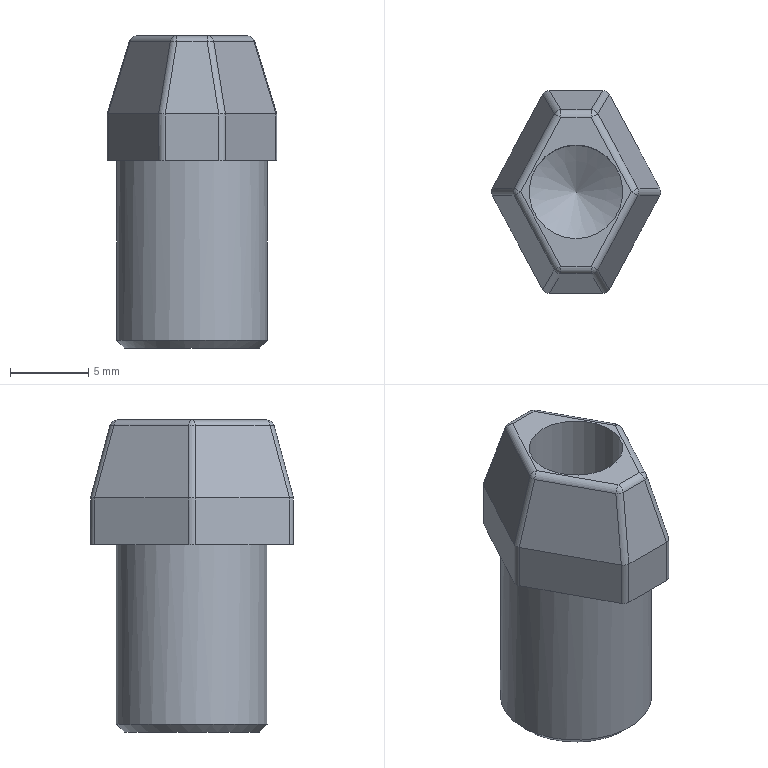Part | NX | features solid 2 | 1 solid | 46 faces | box 10.864 x 13 x 20 mm | volume 1244 mm3 | cylinder 20 | plane 18 | sphere 6 | cone 2 | commonest cylinder face diameters 1 x18 6 x1 9.685 x1
STEP:
#1=CARTESIAN_POINT('',(-137.368,-255.227,120.662));
#2=VERTEX_POINT('',#1);
#3=CARTESIAN_POINT('',(-136.259,-257.286,120.662));
#4=VERTEX_POINT('',#3);
#5=CARTESIAN_POINT('',(-137.495,-254.99,120.662));
#6=DIRECTION('',(0.4741,-0.8805,0.));
#7=VECTOR('',#6,1000.);
#8=LINE('',#5,#7);
#9=EDGE_CURVE('',#2,#4,#8,.T.);
#10=ORIENTED_EDGE('',*,*,#9,.F.);
#11=CARTESIAN_POINT('',(-137.368,-254.753,120.662));
#12=VERTEX_POINT('',#11);
#13=CARTESIAN_POINT('',(-136.927,-254.99,120.662));
#14=DIRECTION('',(0.,0.,1.));
#15=DIRECTION('',(0.,1.,0.));
#16=AXIS2_PLACEMENT_3D('',#13,#14,#15);
#17=CIRCLE('',#16,0.5);
#18=EDGE_CURVE('',#2,#12,#17,.F.);
#19=ORIENTED_EDGE('',*,*,#18,.T.);
#20=CARTESIAN_POINT('',(-136.259,-252.694,120.662));
#21=VERTEX_POINT('',#20);
#22=CARTESIAN_POINT('',(-133.995,-248.49,120.662));
#23=DIRECTION('',(-0.4741,-0.8805,0.));
#24=VECTOR('',#23,1000.);
#25=LINE('',#22,#24);
#26=EDGE_CURVE('',#21,#12,#25,.T.);
#27=ORIENTED_EDGE('',*,*,#26,.F.);
#28=CARTESIAN_POINT('',(-131.995,-254.99,120.662));
#29=DIRECTION('',(0.,0.,1.));
#30=DIRECTION('',(0.,1.,0.));
#31=AXIS2_PLACEMENT_3D('',#28,#29,#30);
#32=CIRCLE('',#31,4.843);
#33=EDGE_CURVE('',#21,#4,#32,.T.);
#34=ORIENTED_EDGE('',*,*,#33,.T.);
#35=EDGE_LOOP('',(#10,#19,#27,#34));
#36=FACE_BOUND('',#35,.T.);
#37=CARTESIAN_POINT('',(-122.995,-261.49,120.662));
#38=DIRECTION('',(0.,0.,1.));
#39=DIRECTION('',(0.,1.,0.));
#40=AXIS2_PLACEMENT_3D('',#37,#38,#39);
#41=PLANE('',#40);
#42=ADVANCED_FACE('',(#36),#41,.F.);
#43=CARTESIAN_POINT('',(-129.854,-261.227,120.662));
#44=VERTEX_POINT('',#43);
#45=CARTESIAN_POINT('',(-127.732,-257.286,120.662));
#46=VERTEX_POINT('',#45);
#47=CARTESIAN_POINT('',(-129.995,-261.49,120.662));
#48=DIRECTION('',(0.4741,0.8805,0.));
#49=VECTOR('',#48,1000.);
#50=LINE('',#47,#49);
#51=EDGE_CURVE('',#44,#46,#50,.T.);
#52=ORIENTED_EDGE('',*,*,#51,.F.);
#53=CARTESIAN_POINT('',(-130.294,-261.49,120.662));
#54=VERTEX_POINT('',#53);
#55=CARTESIAN_POINT('',(-130.294,-260.99,120.662));
#56=DIRECTION('',(0.,0.,1.));
#57=DIRECTION('',(0.,1.,0.));
#58=AXIS2_PLACEMENT_3D('',#55,#56,#57);
#59=CIRCLE('',#58,0.5);
#60=EDGE_CURVE('',#44,#54,#59,.F.);
#61=ORIENTED_EDGE('',*,*,#60,.T.);
#62=CARTESIAN_POINT('',(-133.697,-261.49,120.662));
#63=VERTEX_POINT('',#62);
#64=CARTESIAN_POINT('',(-133.995,-261.49,120.662));
#65=DIRECTION('',(1.,0.,0.));
#66=VECTOR('',#65,1000.);
#67=LINE('',#64,#66);
#68=EDGE_CURVE('',#63,#54,#67,.T.);
#69=ORIENTED_EDGE('',*,*,#68,.F.);
#70=CARTESIAN_POINT('',(-134.137,-261.227,120.662));
#71=VERTEX_POINT('',#70);
#72=CARTESIAN_POINT('',(-133.697,-260.99,120.662));
#73=DIRECTION('',(0.,0.,1.));
#74=DIRECTION('',(0.,1.,0.));
#75=AXIS2_PLACEMENT_3D('',#72,#73,#74);
#76=CIRCLE('',#75,0.5);
#77=EDGE_CURVE('',#63,#71,#76,.F.);
#78=ORIENTED_EDGE('',*,*,#77,.T.);
#79=CARTESIAN_POINT('',(-137.495,-254.99,120.662));
#80=DIRECTION('',(0.4741,-0.8805,0.));
#81=VECTOR('',#80,1000.);
#82=LINE('',#79,#81);
#83=EDGE_CURVE('',#4,#71,#82,.T.);
#84=ORIENTED_EDGE('',*,*,#83,.F.);
#85=CARTESIAN_POINT('',(-131.995,-254.99,120.662));
#86=DIRECTION('',(0.,0.,1.));
#87=DIRECTION('',(0.,1.,0.));
#88=AXIS2_PLACEMENT_3D('',#85,#86,#87);
#89=CIRCLE('',#88,4.843);
#90=EDGE_CURVE('',#4,#46,#89,.T.);
#91=ORIENTED_EDGE('',*,*,#90,.T.);
#92=EDGE_LOOP('',(#52,#61,#69,#78,#84,#91));
#93=FACE_BOUND('',#92,.T.);
#94=CARTESIAN_POINT('',(-122.995,-261.49,120.662));
#95=DIRECTION('',(0.,0.,1.));
#96=DIRECTION('',(0.,1.,0.));
#97=AXIS2_PLACEMENT_3D('',#94,#95,#96);
#98=PLANE('',#97);
#99=ADVANCED_FACE('',(#93),#98,.F.);
#100=CARTESIAN_POINT('',(-126.623,-254.753,120.662));
#101=VERTEX_POINT('',#100);
#102=CARTESIAN_POINT('',(-127.732,-252.694,120.662));
#103=VERTEX_POINT('',#102);
#104=CARTESIAN_POINT('',(-126.495,-254.99,120.662));
#105=DIRECTION('',(-0.4741,0.8805,0.));
#106=VECTOR('',#105,1000.);
#107=LINE('',#104,#106);
#108=EDGE_CURVE('',#101,#103,#107,.T.);
#109=ORIENTED_EDGE('',*,*,#108,.F.);
#110=CARTESIAN_POINT('',(-126.623,-255.227,120.662));
#111=VERTEX_POINT('',#110);
#112=CARTESIAN_POINT('',(-127.063,-254.99,120.662));
#113=DIRECTION('',(0.,0.,1.));
#114=DIRECTION('',(0.,1.,0.));
#115=AXIS2_PLACEMENT_3D('',#112,#113,#114);
#116=CIRCLE('',#115,0.5);
#117=EDGE_CURVE('',#101,#111,#116,.F.);
#118=ORIENTED_EDGE('',*,*,#117,.T.);
#119=CARTESIAN_POINT('',(-129.995,-261.49,120.662));
#120=DIRECTION('',(0.4741,0.8805,0.));
#121=VECTOR('',#120,1000.);
#122=LINE('',#119,#121);
#123=EDGE_CURVE('',#46,#111,#122,.T.);
#124=ORIENTED_EDGE('',*,*,#123,.F.);
#125=CARTESIAN_POINT('',(-131.995,-254.99,120.662));
#126=DIRECTION('',(0.,0.,1.));
#127=DIRECTION('',(0.,1.,0.));
#128=AXIS2_PLACEMENT_3D('',#125,#126,#127);
#129=CIRCLE('',#128,4.843);
#130=EDGE_CURVE('',#46,#103,#129,.T.);
#131=ORIENTED_EDGE('',*,*,#130,.T.);
#132=EDGE_LOOP('',(#109,#118,#124,#131));
#133=FACE_BOUND('',#132,.T.);
#134=CARTESIAN_POINT('',(-122.995,-261.49,120.662));
#135=DIRECTION('',(0.,0.,1.));
#136=DIRECTION('',(0.,1.,0.));
#137=AXIS2_PLACEMENT_3D('',#134,#135,#136);
#138=PLANE('',#137);
#139=ADVANCED_FACE('',(#133),#138,.F.);
#140=ORIENTED_EDGE('',*,*,#68,.T.);
#141=CARTESIAN_POINT('',(-130.294,-261.49,123.662));
#142=VERTEX_POINT('',#141);
#143=CARTESIAN_POINT('',(-130.294,-261.49,123.662));
#144=DIRECTION('',(0.,0.,-1.));
#145=VECTOR('',#144,1000.);
#146=LINE('',#143,#145);
#147=EDGE_CURVE('',#54,#142,#146,.F.);
#148=ORIENTED_EDGE('',*,*,#147,.T.);
#149=CARTESIAN_POINT('',(-133.697,-261.49,123.662));
#150=VERTEX_POINT('',#149);
#151=CARTESIAN_POINT('',(-133.995,-261.49,123.662));
#152=DIRECTION('',(1.,0.,0.));
#153=VECTOR('',#152,1000.);
#154=LINE('',#151,#153);
#155=EDGE_CURVE('',#150,#142,#154,.T.);
#156=ORIENTED_EDGE('',*,*,#155,.F.);
#157=CARTESIAN_POINT('',(-133.697,-261.49,123.662));
#158=DIRECTION('',(0.,0.,-1.));
#159=VECTOR('',#158,1000.);
#160=LINE('',#157,#159);
#161=EDGE_CURVE('',#150,#63,#160,.T.);
#162=ORIENTED_EDGE('',*,*,#161,.T.);
#163=EDGE_LOOP('',(#140,#148,#156,#162));
#164=FACE_BOUND('',#163,.T.);
#165=CARTESIAN_POINT('',(-133.995,-261.49,123.662));
#166=DIRECTION('',(0.,1.,0.));
#167=DIRECTION('',(0.,0.,-1.));
#168=AXIS2_PLACEMENT_3D('',#165,#166,#167);
#169=PLANE('',#168);
#170=ADVANCED_FACE('',(#164),#169,.F.);
#171=ORIENTED_EDGE('',*,*,#123,.T.);
#172=CARTESIAN_POINT('',(-126.623,-255.227,123.662));
#173=VERTEX_POINT('',#172);
#174=CARTESIAN_POINT('',(-126.623,-255.227,123.662));
#175=DIRECTION('',(0.,0.,-1.));
#176=VECTOR('',#175,1000.);
#177=LINE('',#174,#176);
#178=EDGE_CURVE('',#111,#173,#177,.F.);
#179=ORIENTED_EDGE('',*,*,#178,.T.);
#180=CARTESIAN_POINT('',(-129.854,-261.227,123.662));
#181=VERTEX_POINT('',#180);
#182=CARTESIAN_POINT('',(-129.995,-261.49,123.662));
#183=DIRECTION('',(0.4741,0.8805,0.));
#184=VECTOR('',#183,1000.);
#185=LINE('',#182,#184);
#186=EDGE_CURVE('',#181,#173,#185,.T.);
#187=ORIENTED_EDGE('',*,*,#186,.F.);
#188=CARTESIAN_POINT('',(-129.854,-261.227,123.662));
#189=DIRECTION('',(0.,0.,-1.));
#190=VECTOR('',#189,1000.);
#191=LINE('',#188,#190);
#192=EDGE_CURVE('',#181,#44,#191,.T.);
#193=ORIENTED_EDGE('',*,*,#192,.T.);
#194=ORIENTED_EDGE('',*,*,#51,.T.);
#195=EDGE_LOOP('',(#171,#179,#187,#193,#194));
#196=FACE_BOUND('',#195,.T.);
#197=CARTESIAN_POINT('',(-129.995,-261.49,123.662));
#198=DIRECTION('',(-0.8805,0.4741,0.));
#199=DIRECTION('',(-0.4741,-0.8805,0.));
#200=AXIS2_PLACEMENT_3D('',#197,#198,#199);
#201=PLANE('',#200);
#202=ADVANCED_FACE('',(#196),#201,.F.);
#203=CARTESIAN_POINT('',(-129.854,-248.753,120.662));
#204=VERTEX_POINT('',#203);
#205=CARTESIAN_POINT('',(-126.495,-254.99,120.662));
#206=DIRECTION('',(-0.4741,0.8805,0.));
#207=VECTOR('',#206,1000.);
#208=LINE('',#205,#207);
#209=EDGE_CURVE('',#103,#204,#208,.T.);
#210=ORIENTED_EDGE('',*,*,#209,.T.);
#211=CARTESIAN_POINT('',(-129.854,-248.753,123.662));
#212=VERTEX_POINT('',#211);
#213=CARTESIAN_POINT('',(-129.854,-248.753,123.662));
#214=DIRECTION('',(0.,0.,-1.));
#215=VECTOR('',#214,1000.);
#216=LINE('',#213,#215);
#217=EDGE_CURVE('',#204,#212,#216,.F.);
#218=ORIENTED_EDGE('',*,*,#217,.T.);
#219=CARTESIAN_POINT('',(-126.623,-254.753,123.662));
#220=VERTEX_POINT('',#219);
#221=CARTESIAN_POINT('',(-126.495,-254.99,123.662));
#222=DIRECTION('',(-0.4741,0.8805,0.));
#223=VECTOR('',#222,1000.);
#224=LINE('',#221,#223);
#225=EDGE_CURVE('',#220,#212,#224,.T.);
#226=ORIENTED_EDGE('',*,*,#225,.F.);
#227=CARTESIAN_POINT('',(-126.623,-254.753,123.662));
#228=DIRECTION('',(0.,0.,-1.));
#229=VECTOR('',#228,1000.);
#230=LINE('',#227,#229);
#231=EDGE_CURVE('',#220,#101,#230,.T.);
#232=ORIENTED_EDGE('',*,*,#231,.T.);
#233=ORIENTED_EDGE('',*,*,#108,.T.);
#234=EDGE_LOOP('',(#210,#218,#226,#232,#233));
#235=FACE_BOUND('',#234,.T.);
#236=CARTESIAN_POINT('',(-126.495,-254.99,123.662));
#237=DIRECTION('',(-0.8805,-0.4741,0.));
#238=DIRECTION('',(0.4741,-0.8805,0.));
#239=AXIS2_PLACEMENT_3D('',#236,#237,#238);
#240=PLANE('',#239);
#241=ADVANCED_FACE('',(#235),#240,.F.);
#242=CARTESIAN_POINT('',(-130.294,-248.49,123.662));
#243=VERTEX_POINT('',#242);
#244=CARTESIAN_POINT('',(-133.697,-248.49,123.662));
#245=VERTEX_POINT('',#244);
#246=CARTESIAN_POINT('',(-129.995,-248.49,123.662));
#247=DIRECTION('',(-1.,0.,0.));
#248=VECTOR('',#247,1000.);
#249=LINE('',#246,#248);
#250=EDGE_CURVE('',#243,#245,#249,.T.);
#251=ORIENTED_EDGE('',*,*,#250,.F.);
#252=CARTESIAN_POINT('',(-130.294,-248.49,120.662));
#253=VERTEX_POINT('',#252);
#254=CARTESIAN_POINT('',(-130.294,-248.49,123.662));
#255=DIRECTION('',(0.,0.,-1.));
#256=VECTOR('',#255,1000.);
#257=LINE('',#254,#256);
#258=EDGE_CURVE('',#243,#253,#257,.T.);
#259=ORIENTED_EDGE('',*,*,#258,.T.);
#260=CARTESIAN_POINT('',(-133.697,-248.49,120.662));
#261=VERTEX_POINT('',#260);
#262=CARTESIAN_POINT('',(-129.995,-248.49,120.662));
#263=DIRECTION('',(-1.,0.,0.));
#264=VECTOR('',#263,1000.);
#265=LINE('',#262,#264);
#266=EDGE_CURVE('',#253,#261,#265,.T.);
#267=ORIENTED_EDGE('',*,*,#266,.T.);
#268=CARTESIAN_POINT('',(-133.697,-248.49,123.662));
#269=DIRECTION('',(0.,0.,-1.));
#270=VECTOR('',#269,1000.);
#271=LINE('',#268,#270);
#272=EDGE_CURVE('',#261,#245,#271,.F.);
#273=ORIENTED_EDGE('',*,*,#272,.T.);
#274=EDGE_LOOP('',(#251,#259,#267,#273));
#275=FACE_BOUND('',#274,.T.);
#276=CARTESIAN_POINT('',(-129.995,-248.49,123.662));
#277=DIRECTION('',(0.,-1.,0.));
#278=DIRECTION('',(0.,0.,1.));
#279=AXIS2_PLACEMENT_3D('',#276,#277,#278);
#280=PLANE('',#279);
#281=ADVANCED_FACE('',(#275),#280,.F.);
#282=ORIENTED_EDGE('',*,*,#26,.T.);
#283=CARTESIAN_POINT('',(-137.368,-254.753,123.662));
#284=VERTEX_POINT('',#283);
#285=CARTESIAN_POINT('',(-137.368,-254.753,123.662));
#286=DIRECTION('',(0.,0.,-1.));
#287=VECTOR('',#286,1000.);
#288=LINE('',#285,#287);
#289=EDGE_CURVE('',#12,#284,#288,.F.);
#290=ORIENTED_EDGE('',*,*,#289,.T.);
#291=CARTESIAN_POINT('',(-134.137,-248.753,123.662));
#292=VERTEX_POINT('',#291);
#293=CARTESIAN_POINT('',(-133.995,-248.49,123.662));
#294=DIRECTION('',(-0.4741,-0.8805,0.));
#295=VECTOR('',#294,1000.);
#296=LINE('',#293,#295);
#297=EDGE_CURVE('',#292,#284,#296,.T.);
#298=ORIENTED_EDGE('',*,*,#297,.F.);
#299=CARTESIAN_POINT('',(-134.137,-248.753,120.662));
#300=VERTEX_POINT('',#299);
#301=CARTESIAN_POINT('',(-134.137,-248.753,123.662));
#302=DIRECTION('',(0.,0.,-1.));
#303=VECTOR('',#302,1000.);
#304=LINE('',#301,#303);
#305=EDGE_CURVE('',#292,#300,#304,.T.);
#306=ORIENTED_EDGE('',*,*,#305,.T.);
#307=CARTESIAN_POINT('',(-133.995,-248.49,120.662));
#308=DIRECTION('',(-0.4741,-0.8805,0.));
#309=VECTOR('',#308,1000.);
#310=LINE('',#307,#309);
#311=EDGE_CURVE('',#300,#21,#310,.T.);
#312=ORIENTED_EDGE('',*,*,#311,.T.);
#313=EDGE_LOOP('',(#282,#290,#298,#306,#312));
#314=FACE_BOUND('',#313,.T.);
#315=CARTESIAN_POINT('',(-133.995,-248.49,123.662));
#316=DIRECTION('',(0.8805,-0.4741,0.));
#317=DIRECTION('',(0.4741,0.8805,0.));
#318=AXIS2_PLACEMENT_3D('',#315,#316,#317);
#319=PLANE('',#318);
#320=ADVANCED_FACE('',(#314),#319,.F.);
#321=ORIENTED_EDGE('',*,*,#83,.T.);
#322=CARTESIAN_POINT('',(-134.137,-261.227,123.662));
#323=VERTEX_POINT('',#322);
#324=CARTESIAN_POINT('',(-134.137,-261.227,123.662));
#325=DIRECTION('',(0.,0.,-1.));
#326=VECTOR('',#325,1000.);
#327=LINE('',#324,#326);
#328=EDGE_CURVE('',#71,#323,#327,.F.);
#329=ORIENTED_EDGE('',*,*,#328,.T.);
#330=CARTESIAN_POINT('',(-137.368,-255.227,123.662));
#331=VERTEX_POINT('',#330);
#332=CARTESIAN_POINT('',(-137.495,-254.99,123.662));
#333=DIRECTION('',(0.4741,-0.8805,0.));
#334=VECTOR('',#333,1000.);
#335=LINE('',#332,#334);
#336=EDGE_CURVE('',#331,#323,#335,.T.);
#337=ORIENTED_EDGE('',*,*,#336,.F.);
#338=CARTESIAN_POINT('',(-137.368,-255.227,123.662));
#339=DIRECTION('',(0.,0.,-1.));
#340=VECTOR('',#339,1000.);
#341=LINE('',#338,#340);
#342=EDGE_CURVE('',#331,#2,#341,.T.);
#343=ORIENTED_EDGE('',*,*,#342,.T.);
#344=ORIENTED_EDGE('',*,*,#9,.T.);
#345=EDGE_LOOP('',(#321,#329,#337,#343,#344));
#346=FACE_BOUND('',#345,.T.);
#347=CARTESIAN_POINT('',(-137.495,-254.99,123.662));
#348=DIRECTION('',(0.8805,0.4741,0.));
#349=DIRECTION('',(-0.4741,0.8805,0.));
#350=AXIS2_PLACEMENT_3D('',#347,#348,#349);
#351=PLANE('',#350);
#352=ADVANCED_FACE('',(#346),#351,.F.);
#353=ORIENTED_EDGE('',*,*,#266,.F.);
#354=CARTESIAN_POINT('',(-130.294,-248.99,120.662));
#355=DIRECTION('',(0.,0.,1.));
#356=DIRECTION('',(0.,1.,0.));
#357=AXIS2_PLACEMENT_3D('',#354,#355,#356);
#358=CIRCLE('',#357,0.5);
#359=EDGE_CURVE('',#253,#204,#358,.F.);
#360=ORIENTED_EDGE('',*,*,#359,.T.);
#361=ORIENTED_EDGE('',*,*,#209,.F.);
#362=CARTESIAN_POINT('',(-131.995,-254.99,120.662));
#363=DIRECTION('',(0.,0.,1.));
#364=DIRECTION('',(0.,1.,0.));
#365=AXIS2_PLACEMENT_3D('',#362,#363,#364);
#366=CIRCLE('',#365,4.843);
#367=EDGE_CURVE('',#103,#21,#366,.T.);
#368=ORIENTED_EDGE('',*,*,#367,.T.);
#369=ORIENTED_EDGE('',*,*,#311,.F.);
#370=CARTESIAN_POINT('',(-133.697,-248.99,120.662));
#371=DIRECTION('',(0.,0.,1.));
#372=DIRECTION('',(0.,1.,0.));
#373=AXIS2_PLACEMENT_3D('',#370,#371,#372);
#374=CIRCLE('',#373,0.5);
#375=EDGE_CURVE('',#300,#261,#374,.F.);
#376=ORIENTED_EDGE('',*,*,#375,.T.);
#377=EDGE_LOOP('',(#353,#360,#361,#368,#369,#376));
#378=FACE_BOUND('',#377,.T.);
#379=CARTESIAN_POINT('',(-122.995,-261.49,120.662));
#380=DIRECTION('',(0.,0.,1.));
#381=DIRECTION('',(0.,1.,0.));
#382=AXIS2_PLACEMENT_3D('',#379,#380,#381);
#383=PLANE('',#382);
#384=ADVANCED_FACE('',(#378),#383,.F.);
#385=ORIENTED_EDGE('',*,*,#336,.T.);
#386=CARTESIAN_POINT('',(-134.132,-261.236,123.663));
#387=VERTEX_POINT('',#386);
#388=CARTESIAN_POINT('',(-133.697,-260.99,125.528));
#389=DIRECTION('',(-0.8505,-0.4579,0.2588));
#390=DIRECTION('',(-0.2279,-0.1227,-0.9659));
#391=AXIS2_PLACEMENT_3D('',#388,#389,#390);
#392=ELLIPSE('',#391,1.932,0.5);
#393=EDGE_CURVE('',#323,#387,#392,.T.);
#394=ORIENTED_EDGE('',*,*,#393,.T.);
#395=CARTESIAN_POINT('',(-133.391,-259.996,128.292));
#396=VERTEX_POINT('',#395);
#397=CARTESIAN_POINT('',(-134.027,-261.061,124.317));
#398=DIRECTION('',(0.1528,0.2558,0.9546));
#399=VECTOR('',#398,1000.);
#400=LINE('',#397,#399);
#401=EDGE_CURVE('',#387,#396,#400,.T.);
#402=ORIENTED_EDGE('',*,*,#401,.T.);
#403=CARTESIAN_POINT('',(-135.963,-255.219,128.292));
#404=VERTEX_POINT('',#403);
#405=CARTESIAN_POINT('',(-136.061,-255.037,128.292));
#406=DIRECTION('',(0.4741,-0.8805,0.));
#407=VECTOR('',#406,1000.);
#408=LINE('',#405,#407);
#409=EDGE_CURVE('',#396,#404,#408,.F.);
#410=ORIENTED_EDGE('',*,*,#409,.T.);
#411=CARTESIAN_POINT('',(-137.372,-255.219,123.663));
#412=VERTEX_POINT('',#411);
#413=CARTESIAN_POINT('',(-137.278,-255.219,123.972));
#414=DIRECTION('',(0.2911,0.,0.9567));
#415=VECTOR('',#414,1000.);
#416=LINE('',#413,#415);
#417=EDGE_CURVE('',#404,#412,#416,.F.);
#418=ORIENTED_EDGE('',*,*,#417,.T.);
#419=CARTESIAN_POINT('',(-136.927,-254.99,125.528));
#420=DIRECTION('',(-0.8505,-0.4579,0.2588));
#421=DIRECTION('',(-0.2279,-0.1227,-0.9659));
#422=AXIS2_PLACEMENT_3D('',#419,#420,#421);
#423=ELLIPSE('',#422,1.932,0.5);
#424=EDGE_CURVE('',#412,#331,#423,.T.);
#425=ORIENTED_EDGE('',*,*,#424,.T.);
#426=EDGE_LOOP('',(#385,#394,#402,#410,#418,#425));
#427=FACE_BOUND('',#426,.T.);
#428=CARTESIAN_POINT('',(-136.259,-257.286,123.662));
#429=DIRECTION('',(-0.8505,-0.4579,0.2588));
#430=DIRECTION('',(0.4741,-0.8805,0.));
#431=AXIS2_PLACEMENT_3D('',#428,#429,#430);
#432=PLANE('',#431);
#433=ADVANCED_FACE('',(#427),#432,.T.);
#434=ORIENTED_EDGE('',*,*,#155,.T.);
#435=CARTESIAN_POINT('',(-130.284,-261.49,123.663));
#436=VERTEX_POINT('',#435);
#437=CARTESIAN_POINT('',(-130.294,-260.99,125.528));
#438=DIRECTION('',(0.,-0.9659,0.2588));
#439=DIRECTION('',(0.,-0.2588,-0.9659));
#440=AXIS2_PLACEMENT_3D('',#437,#438,#439);
#441=ELLIPSE('',#440,1.932,0.5);
#442=EDGE_CURVE('',#142,#436,#441,.T.);
#443=ORIENTED_EDGE('',*,*,#442,.T.);
#444=CARTESIAN_POINT('',(-131.025,-260.25,128.292));
#445=VERTEX_POINT('',#444);
#446=CARTESIAN_POINT('',(-130.324,-261.423,123.912));
#447=DIRECTION('',(-0.1528,0.2558,0.9546));
#448=VECTOR('',#447,1000.);
#449=LINE('',#446,#448);
#450=EDGE_CURVE('',#436,#445,#449,.T.);
#451=ORIENTED_EDGE('',*,*,#450,.T.);
#452=CARTESIAN_POINT('',(-132.966,-260.25,128.292));
#453=VERTEX_POINT('',#452);
#454=CARTESIAN_POINT('',(-133.195,-260.25,128.292));
#455=DIRECTION('',(1.,0.,0.));
#456=VECTOR('',#455,1000.);
#457=LINE('',#454,#456);
#458=EDGE_CURVE('',#445,#453,#457,.F.);
#459=ORIENTED_EDGE('',*,*,#458,.T.);
#460=CARTESIAN_POINT('',(-133.707,-261.49,123.663));
#461=VERTEX_POINT('',#460);
#462=CARTESIAN_POINT('',(-133.667,-261.423,123.912));
#463=DIRECTION('',(0.1528,0.2558,0.9546));
#464=VECTOR('',#463,1000.);
#465=LINE('',#462,#464);
#466=EDGE_CURVE('',#453,#461,#465,.F.);
#467=ORIENTED_EDGE('',*,*,#466,.T.);
#468=CARTESIAN_POINT('',(-133.697,-260.99,125.528));
#469=DIRECTION('',(0.,-0.9659,0.2588));
#470=DIRECTION('',(0.,-0.2588,-0.9659));
#471=AXIS2_PLACEMENT_3D('',#468,#469,#470);
#472=ELLIPSE('',#471,1.932,0.5);
#473=EDGE_CURVE('',#461,#150,#472,.T.);
#474=ORIENTED_EDGE('',*,*,#473,.T.);
#475=EDGE_LOOP('',(#434,#443,#451,#459,#467,#474));
#476=FACE_BOUND('',#475,.T.);
#477=CARTESIAN_POINT('',(-131.995,-261.49,123.662));
#478=DIRECTION('',(0.,-0.9659,0.2588));
#479=DIRECTION('',(0.,0.2588,0.9659));
#480=AXIS2_PLACEMENT_3D('',#477,#478,#479);
#481=PLANE('',#480);
#482=ADVANCED_FACE('',(#476),#481,.T.);
#483=ORIENTED_EDGE('',*,*,#186,.T.);
#484=CARTESIAN_POINT('',(-126.619,-255.219,123.663));
#485=VERTEX_POINT('',#484);
#486=CARTESIAN_POINT('',(-127.063,-254.99,125.528));
#487=DIRECTION('',(0.8505,-0.4579,0.2588));
#488=DIRECTION('',(0.2279,-0.1227,-0.9659));
#489=AXIS2_PLACEMENT_3D('',#486,#487,#488);
#490=ELLIPSE('',#489,1.932,0.5);
#491=EDGE_CURVE('',#173,#485,#490,.T.);
#492=ORIENTED_EDGE('',*,*,#491,.T.);
#493=CARTESIAN_POINT('',(-128.027,-255.219,128.292));
#494=VERTEX_POINT('',#493);
#495=CARTESIAN_POINT('',(-126.713,-255.219,123.972));
#496=DIRECTION('',(-0.2911,0.,0.9567));
#497=VECTOR('',#496,1000.);
#498=LINE('',#495,#497);
#499=EDGE_CURVE('',#485,#494,#498,.T.);
#500=ORIENTED_EDGE('',*,*,#499,.T.);
#501=CARTESIAN_POINT('',(-130.599,-259.996,128.292));
#502=VERTEX_POINT('',#501);
#503=CARTESIAN_POINT('',(-130.708,-260.198,128.292));
#504=DIRECTION('',(0.4741,0.8805,0.));
#505=VECTOR('',#504,1000.);
#506=LINE('',#503,#505);
#507=EDGE_CURVE('',#494,#502,#506,.F.);
#508=ORIENTED_EDGE('',*,*,#507,.T.);
#509=CARTESIAN_POINT('',(-129.859,-261.236,123.663));
#510=VERTEX_POINT('',#509);
#511=CARTESIAN_POINT('',(-129.963,-261.061,124.317));
#512=DIRECTION('',(-0.1528,0.2558,0.9546));
#513=VECTOR('',#512,1000.);
#514=LINE('',#511,#513);
#515=EDGE_CURVE('',#502,#510,#514,.F.);
#516=ORIENTED_EDGE('',*,*,#515,.T.);
#517=CARTESIAN_POINT('',(-130.294,-260.99,125.528));
#518=DIRECTION('',(0.8505,-0.4579,0.2588));
#519=DIRECTION('',(0.2279,-0.1227,-0.9659));
#520=AXIS2_PLACEMENT_3D('',#517,#518,#519);
#521=ELLIPSE('',#520,1.932,0.5);
#522=EDGE_CURVE('',#510,#181,#521,.T.);
#523=ORIENTED_EDGE('',*,*,#522,.T.);
#524=EDGE_LOOP('',(#483,#492,#500,#508,#516,#523));
#525=FACE_BOUND('',#524,.T.);
#526=CARTESIAN_POINT('',(-127.732,-257.286,123.662));
#527=DIRECTION('',(0.8505,-0.4579,0.2588));
#528=DIRECTION('',(0.4741,0.8805,0.));
#529=AXIS2_PLACEMENT_3D('',#526,#527,#528);
#530=PLANE('',#529);
#531=ADVANCED_FACE('',(#525),#530,.T.);
#532=ORIENTED_EDGE('',*,*,#225,.T.);
#533=CARTESIAN_POINT('',(-129.859,-248.744,123.663));
#534=VERTEX_POINT('',#533);
#535=CARTESIAN_POINT('',(-130.294,-248.99,125.528));
#536=DIRECTION('',(0.8505,0.4579,0.2588));
#537=DIRECTION('',(0.2279,0.1227,-0.9659));
#538=AXIS2_PLACEMENT_3D('',#535,#536,#537);
#539=ELLIPSE('',#538,1.932,0.5);
#540=EDGE_CURVE('',#212,#534,#539,.T.);
#541=ORIENTED_EDGE('',*,*,#540,.T.);
#542=CARTESIAN_POINT('',(-130.599,-249.985,128.292));
#543=VERTEX_POINT('',#542);
#544=CARTESIAN_POINT('',(-129.963,-248.92,124.317));
#545=DIRECTION('',(-0.1528,-0.2558,0.9546));
#546=VECTOR('',#545,1000.);
#547=LINE('',#544,#546);
#548=EDGE_CURVE('',#534,#543,#547,.T.);
#549=ORIENTED_EDGE('',*,*,#548,.T.);
#550=CARTESIAN_POINT('',(-128.027,-254.761,128.292));
#551=VERTEX_POINT('',#550);
#552=CARTESIAN_POINT('',(-127.929,-254.943,128.292));
#553=DIRECTION('',(-0.4741,0.8805,0.));
#554=VECTOR('',#553,1000.);
#555=LINE('',#552,#554);
#556=EDGE_CURVE('',#543,#551,#555,.F.);
#557=ORIENTED_EDGE('',*,*,#556,.T.);
#558=CARTESIAN_POINT('',(-126.619,-254.761,123.663));
#559=VERTEX_POINT('',#558);
#560=CARTESIAN_POINT('',(-126.713,-254.761,123.972));
#561=DIRECTION('',(-0.2911,0.,0.9567));
#562=VECTOR('',#561,1000.);
#563=LINE('',#560,#562);
#564=EDGE_CURVE('',#551,#559,#563,.F.);
#565=ORIENTED_EDGE('',*,*,#564,.T.);
#566=CARTESIAN_POINT('',(-127.063,-254.99,125.528));
#567=DIRECTION('',(0.8505,0.4579,0.2588));
#568=DIRECTION('',(0.2279,0.1227,-0.9659));
#569=AXIS2_PLACEMENT_3D('',#566,#567,#568);
#570=ELLIPSE('',#569,1.932,0.5);
#571=EDGE_CURVE('',#559,#220,#570,.T.);
#572=ORIENTED_EDGE('',*,*,#571,.T.);
#573=EDGE_LOOP('',(#532,#541,#549,#557,#565,#572));
#574=FACE_BOUND('',#573,.T.);
#575=CARTESIAN_POINT('',(-127.732,-252.694,123.662));
#576=DIRECTION('',(0.8505,0.4579,0.2588));
#577=DIRECTION('',(-0.4741,0.8805,0.));
#578=AXIS2_PLACEMENT_3D('',#575,#576,#577);
#579=PLANE('',#578);
#580=ADVANCED_FACE('',(#574),#579,.T.);
#581=CARTESIAN_POINT('',(-131.025,-249.731,128.292));
#582=VERTEX_POINT('',#581);
#583=CARTESIAN_POINT('',(-130.284,-248.49,123.663));
#584=VERTEX_POINT('',#583);
#585=CARTESIAN_POINT('',(-130.324,-248.557,123.912));
#586=DIRECTION('',(-0.1528,-0.2558,0.9546));
#587=VECTOR('',#586,1000.);
#588=LINE('',#585,#587);
#589=EDGE_CURVE('',#582,#584,#588,.F.);
#590=ORIENTED_EDGE('',*,*,#589,.T.);
#591=CARTESIAN_POINT('',(-130.294,-248.99,125.528));
#592=DIRECTION('',(0.,0.9659,0.2588));
#593=DIRECTION('',(0.,0.2588,-0.9659));
#594=AXIS2_PLACEMENT_3D('',#591,#592,#593);
#595=ELLIPSE('',#594,1.932,0.5);
#596=EDGE_CURVE('',#584,#243,#595,.T.);
#597=ORIENTED_EDGE('',*,*,#596,.T.);
#598=ORIENTED_EDGE('',*,*,#250,.T.);
#599=CARTESIAN_POINT('',(-133.707,-248.49,123.663));
#600=VERTEX_POINT('',#599);
#601=CARTESIAN_POINT('',(-133.697,-248.99,125.528));
#602=DIRECTION('',(0.,0.9659,0.2588));
#603=DIRECTION('',(0.,0.2588,-0.9659));
#604=AXIS2_PLACEMENT_3D('',#601,#602,#603);
#605=ELLIPSE('',#604,1.932,0.5);
#606=EDGE_CURVE('',#245,#600,#605,.T.);
#607=ORIENTED_EDGE('',*,*,#606,.T.);
#608=CARTESIAN_POINT('',(-132.966,-249.731,128.292));
#609=VERTEX_POINT('',#608);
#610=CARTESIAN_POINT('',(-133.667,-248.557,123.912));
#611=DIRECTION('',(0.1528,-0.2558,0.9546));
#612=VECTOR('',#611,1000.);
#613=LINE('',#610,#612);
#614=EDGE_CURVE('',#600,#609,#613,.T.);
#615=ORIENTED_EDGE('',*,*,#614,.T.);
#616=CARTESIAN_POINT('',(-130.796,-249.731,128.292));
#617=DIRECTION('',(-1.,0.,0.));
#618=VECTOR('',#617,1000.);
#619=LINE('',#616,#618);
#620=EDGE_CURVE('',#609,#582,#619,.F.);
#621=ORIENTED_EDGE('',*,*,#620,.T.);
#622=EDGE_LOOP('',(#590,#597,#598,#607,#615,#621));
#623=FACE_BOUND('',#622,.T.);
#624=CARTESIAN_POINT('',(-131.995,-248.49,123.662));
#625=DIRECTION('',(0.,0.9659,0.2588));
#626=DIRECTION('',(0.,0.2588,-0.9659));
#627=AXIS2_PLACEMENT_3D('',#624,#625,#626);
#628=PLANE('',#627);
#629=ADVANCED_FACE('',(#623),#628,.T.);
#630=ORIENTED_EDGE('',*,*,#297,.T.);
#631=CARTESIAN_POINT('',(-137.372,-254.761,123.663));
#632=VERTEX_POINT('',#631);
#633=CARTESIAN_POINT('',(-136.927,-254.99,125.528));
#634=DIRECTION('',(-0.8505,0.4579,0.2588));
#635=DIRECTION('',(-0.2279,0.1227,-0.9659));
#636=AXIS2_PLACEMENT_3D('',#633,#634,#635);
#637=ELLIPSE('',#636,1.932,0.5);
#638=EDGE_CURVE('',#284,#632,#637,.T.);
#639=ORIENTED_EDGE('',*,*,#638,.T.);
#640=CARTESIAN_POINT('',(-135.963,-254.761,128.292));
#641=VERTEX_POINT('',#640);
#642=CARTESIAN_POINT('',(-137.278,-254.761,123.972));
#643=DIRECTION('',(0.2911,0.,0.9567));
#644=VECTOR('',#643,1000.);
#645=LINE('',#642,#644);
#646=EDGE_CURVE('',#632,#641,#645,.T.);
#647=ORIENTED_EDGE('',*,*,#646,.T.);
#648=CARTESIAN_POINT('',(-133.391,-249.985,128.292));
#649=VERTEX_POINT('',#648);
#650=CARTESIAN_POINT('',(-133.282,-249.783,128.292));
#651=DIRECTION('',(-0.4741,-0.8805,0.));
#652=VECTOR('',#651,1000.);
#653=LINE('',#650,#652);
#654=EDGE_CURVE('',#641,#649,#653,.F.);
#655=ORIENTED_EDGE('',*,*,#654,.T.);
#656=CARTESIAN_POINT('',(-134.132,-248.744,123.663));
#657=VERTEX_POINT('',#656);
#658=CARTESIAN_POINT('',(-134.027,-248.92,124.317));
#659=DIRECTION('',(0.1528,-0.2558,0.9546));
#660=VECTOR('',#659,1000.);
#661=LINE('',#658,#660);
#662=EDGE_CURVE('',#649,#657,#661,.F.);
#663=ORIENTED_EDGE('',*,*,#662,.T.);
#664=CARTESIAN_POINT('',(-133.697,-248.99,125.528));
#665=DIRECTION('',(-0.8505,0.4579,0.2588));
#666=DIRECTION('',(-0.2279,0.1227,-0.9659));
#667=AXIS2_PLACEMENT_3D('',#664,#665,#666);
#668=ELLIPSE('',#667,1.932,0.5);
#669=EDGE_CURVE('',#657,#292,#668,.T.);
#670=ORIENTED_EDGE('',*,*,#669,.T.);
#671=EDGE_LOOP('',(#630,#639,#647,#655,#663,#670));
#672=FACE_BOUND('',#671,.T.);
#673=CARTESIAN_POINT('',(-136.259,-252.694,123.662));
#674=DIRECTION('',(-0.8505,0.4579,0.2588));
#675=DIRECTION('',(-0.4741,-0.8805,0.));
#676=AXIS2_PLACEMENT_3D('',#673,#674,#675);
#677=PLANE('',#676);
#678=ADVANCED_FACE('',(#672),#677,.T.);
#679=CARTESIAN_POINT('',(-131.025,-259.767,128.662));
#680=VERTEX_POINT('',#679);
#681=CARTESIAN_POINT('',(-128.453,-254.99,128.662));
#682=VERTEX_POINT('',#681);
#683=CARTESIAN_POINT('',(-128.355,-254.808,128.662));
#684=DIRECTION('',(-0.4741,-0.8805,0.));
#685=VECTOR('',#684,1000.);
#686=LINE('',#683,#685);
#687=EDGE_CURVE('',#680,#682,#686,.F.);
#688=ORIENTED_EDGE('',*,*,#687,.T.);
#689=CARTESIAN_POINT('',(-131.025,-250.214,128.662));
#690=VERTEX_POINT('',#689);
#691=CARTESIAN_POINT('',(-131.133,-250.012,128.662));
#692=DIRECTION('',(0.4741,-0.8805,0.));
#693=VECTOR('',#692,1000.);
#694=LINE('',#691,#693);
#695=EDGE_CURVE('',#682,#690,#694,.F.);
#696=ORIENTED_EDGE('',*,*,#695,.T.);
#697=CARTESIAN_POINT('',(-132.966,-250.214,128.662));
#698=VERTEX_POINT('',#697);
#699=CARTESIAN_POINT('',(-133.195,-250.214,128.662));
#700=DIRECTION('',(1.,0.,0.));
#701=VECTOR('',#700,1000.);
#702=LINE('',#699,#701);
#703=EDGE_CURVE('',#690,#698,#702,.F.);
#704=ORIENTED_EDGE('',*,*,#703,.T.);
#705=CARTESIAN_POINT('',(-135.538,-254.99,128.662));
#706=VERTEX_POINT('',#705);
#707=CARTESIAN_POINT('',(-135.636,-255.172,128.662));
#708=DIRECTION('',(0.4741,0.8805,0.));
#709=VECTOR('',#708,1000.);
#710=LINE('',#707,#709);
#711=EDGE_CURVE('',#698,#706,#710,.F.);
#712=ORIENTED_EDGE('',*,*,#711,.T.);
#713=CARTESIAN_POINT('',(-132.966,-259.767,128.662));
#714=VERTEX_POINT('',#713);
#715=CARTESIAN_POINT('',(-132.857,-259.969,128.662));
#716=DIRECTION('',(-0.4741,0.8805,0.));
#717=VECTOR('',#716,1000.);
#718=LINE('',#715,#717);
#719=EDGE_CURVE('',#706,#714,#718,.F.);
#720=ORIENTED_EDGE('',*,*,#719,.T.);
#721=CARTESIAN_POINT('',(-130.796,-259.767,128.662));
#722=DIRECTION('',(-1.,0.,0.));
#723=VECTOR('',#722,1000.);
#724=LINE('',#721,#723);
#725=EDGE_CURVE('',#714,#680,#724,.F.);
#726=ORIENTED_EDGE('',*,*,#725,.T.);
#727=EDGE_LOOP('',(#688,#696,#704,#712,#720,#726));
#728=FACE_BOUND('',#727,.T.);
#729=CARTESIAN_POINT('',(-131.995,-257.99,128.662));
#730=VERTEX_POINT('',#729);
#731=CARTESIAN_POINT('',(-131.995,-254.99,128.662));
#732=DIRECTION('',(0.,0.,-1.));
#733=DIRECTION('',(0.,-1.,0.));
#734=AXIS2_PLACEMENT_3D('',#731,#732,#733);
#735=CIRCLE('',#734,3.);
#736=EDGE_CURVE('',#730,#730,#735,.T.);
#737=ORIENTED_EDGE('',*,*,#736,.T.);
#738=EDGE_LOOP('',(#737));
#739=FACE_BOUND('',#738,.T.);
#740=CARTESIAN_POINT('',(-133.995,-261.49,128.662));
#741=DIRECTION('',(0.,0.,1.));
#742=DIRECTION('',(0.,1.,0.));
#743=AXIS2_PLACEMENT_3D('',#740,#741,#742);
#744=PLANE('',#743);
#745=ADVANCED_FACE('',(#728,#739),#744,.T.);
#746=CARTESIAN_POINT('',(-131.995,-250.148,109.162));
#747=VERTEX_POINT('',#746);
#748=CARTESIAN_POINT('',(-131.995,-254.99,109.162));
#749=DIRECTION('',(0.,0.,1.));
#750=DIRECTION('',(0.,1.,0.));
#751=AXIS2_PLACEMENT_3D('',#748,#749,#750);
#752=CIRCLE('',#751,4.843);
#753=EDGE_CURVE('',#747,#747,#752,.T.);
#754=ORIENTED_EDGE('',*,*,#753,.T.);
#755=EDGE_LOOP('',(#754));
#756=FACE_BOUND('',#755,.T.);
#757=ORIENTED_EDGE('',*,*,#33,.F.);
#758=ORIENTED_EDGE('',*,*,#367,.F.);
#759=ORIENTED_EDGE('',*,*,#130,.F.);
#760=ORIENTED_EDGE('',*,*,#90,.F.);
#761=EDGE_LOOP('',(#757,#758,#759,#760));
#762=FACE_BOUND('',#761,.T.);
#763=CARTESIAN_POINT('',(-131.995,-254.99,108.662));
#764=DIRECTION('',(0.,0.,1.));
#765=DIRECTION('',(0.,1.,0.));
#766=AXIS2_PLACEMENT_3D('',#763,#764,#765);
#767=CYLINDRICAL_SURFACE('',#766,4.843);
#768=ADVANCED_FACE('',(#756,#762),#767,.T.);
#769=CARTESIAN_POINT('',(-131.995,-250.648,108.662));
#770=VERTEX_POINT('',#769);
#771=CARTESIAN_POINT('',(-131.995,-254.99,108.662));
#772=DIRECTION('',(0.,0.,1.));
#773=DIRECTION('',(0.,1.,0.));
#774=AXIS2_PLACEMENT_3D('',#771,#772,#773);
#775=CIRCLE('',#774,4.343);
#776=EDGE_CURVE('',#770,#770,#775,.F.);
#777=ORIENTED_EDGE('',*,*,#776,.T.);
#778=EDGE_LOOP('',(#777));
#779=FACE_BOUND('',#778,.T.);
#780=CARTESIAN_POINT('',(-131.995,-254.99,108.662));
#781=DIRECTION('',(0.,0.,1.));
#782=DIRECTION('',(0.,1.,0.));
#783=AXIS2_PLACEMENT_3D('',#780,#781,#782);
#784=PLANE('',#783);
#785=ADVANCED_FACE('',(#779),#784,.F.);
#786=ORIENTED_EDGE('',*,*,#776,.F.);
#787=EDGE_LOOP('',(#786));
#788=FACE_BOUND('',#787,.T.);
#789=ORIENTED_EDGE('',*,*,#753,.F.);
#790=EDGE_LOOP('',(#789));
#791=FACE_BOUND('',#790,.T.);
#792=CARTESIAN_POINT('',(-131.995,-254.99,109.162));
#793=DIRECTION('',(0.,0.,1.));
#794=DIRECTION('',(0.,1.,0.));
#795=AXIS2_PLACEMENT_3D('',#792,#793,#794);
#796=CONICAL_SURFACE('',#795,4.843,0.7854);
#797=ADVANCED_FACE('',(#788,#791),#796,.T.);
#798=CARTESIAN_POINT('',(-131.995,-257.99,118.662));
#799=VERTEX_POINT('',#798);
#800=CARTESIAN_POINT('',(-131.995,-254.99,118.662));
#801=DIRECTION('',(0.,0.,-1.));
#802=DIRECTION('',(0.,-1.,0.));
#803=AXIS2_PLACEMENT_3D('',#800,#801,#802);
#804=CIRCLE('',#803,3.);
#805=EDGE_CURVE('',#799,#799,#804,.T.);
#806=ORIENTED_EDGE('',*,*,#805,.F.);
#807=EDGE_LOOP('',(#806));
#808=FACE_BOUND('',#807,.T.);
#809=CARTESIAN_POINT('',(-131.995,-254.99,116.86));
#810=VERTEX_POINT('',#809);
#811=VERTEX_LOOP('',#810);
#812=FACE_BOUND('',#811,.T.);
#813=CARTESIAN_POINT('',(-131.995,-254.99,118.662));
#814=DIRECTION('',(0.,0.,1.));
#815=DIRECTION('',(0.,1.,0.));
#816=AXIS2_PLACEMENT_3D('',#813,#814,#815);
#817=CONICAL_SURFACE('',#816,3.,1.03);
#818=ADVANCED_FACE('',(#808,#812),#817,.F.);
#819=ORIENTED_EDGE('',*,*,#805,.T.);
#820=EDGE_LOOP('',(#819));
#821=FACE_BOUND('',#820,.T.);
#822=ORIENTED_EDGE('',*,*,#736,.F.);
#823=EDGE_LOOP('',(#822));
#824=FACE_BOUND('',#823,.T.);
#825=CARTESIAN_POINT('',(-131.995,-254.99,128.662));
#826=DIRECTION('',(0.,0.,-1.));
#827=DIRECTION('',(0.,-1.,0.));
#828=AXIS2_PLACEMENT_3D('',#825,#826,#827);
#829=CYLINDRICAL_SURFACE('',#828,3.);
#830=ADVANCED_FACE('',(#821,#824),#829,.F.);
#831=ORIENTED_EDGE('',*,*,#161,.F.);
#832=ORIENTED_EDGE('',*,*,#473,.F.);
#833=CARTESIAN_POINT('',(-133.697,-260.99,123.597));
#834=DIRECTION('',(-0.07727,-0.1294,-0.9886));
#835=DIRECTION('',(-0.5069,-0.8487,0.1507));
#836=AXIS2_PLACEMENT_3D('',#833,#834,#835);
#837=ELLIPSE('',#836,0.5058,0.5);
#838=EDGE_CURVE('',#387,#461,#837,.F.);
#839=ORIENTED_EDGE('',*,*,#838,.F.);
#840=ORIENTED_EDGE('',*,*,#393,.F.);
#841=ORIENTED_EDGE('',*,*,#328,.F.);
#842=ORIENTED_EDGE('',*,*,#77,.F.);
#843=EDGE_LOOP('',(#831,#832,#839,#840,#841,#842));
#844=FACE_BOUND('',#843,.T.);
#845=CARTESIAN_POINT('',(-133.697,-260.99,123.662));
#846=DIRECTION('',(0.,0.,-1.));
#847=DIRECTION('',(0.,-1.,0.));
#848=AXIS2_PLACEMENT_3D('',#845,#846,#847);
#849=CYLINDRICAL_SURFACE('',#848,0.5);
#850=ADVANCED_FACE('',(#844),#849,.T.);
#851=ORIENTED_EDGE('',*,*,#838,.T.);
#852=ORIENTED_EDGE('',*,*,#466,.F.);
#853=CARTESIAN_POINT('',(-132.966,-259.767,128.162));
#854=DIRECTION('',(0.1528,0.2558,0.9546));
#855=DIRECTION('',(0.,0.9659,-0.2588));
#856=AXIS2_PLACEMENT_3D('',#853,#854,#855);
#857=CIRCLE('',#856,0.5);
#858=EDGE_CURVE('',#396,#453,#857,.T.);
#859=ORIENTED_EDGE('',*,*,#858,.F.);
#860=ORIENTED_EDGE('',*,*,#401,.F.);
#861=EDGE_LOOP('',(#851,#852,#859,#860));
#862=FACE_BOUND('',#861,.T.);
#863=CARTESIAN_POINT('',(-133.667,-260.941,123.783));
#864=DIRECTION('',(-0.1528,-0.2558,-0.9546));
#865=DIRECTION('',(0.,-0.9659,0.2588));
#866=AXIS2_PLACEMENT_3D('',#863,#864,#865);
#867=CYLINDRICAL_SURFACE('',#866,0.5);
#868=ADVANCED_FACE('',(#862),#867,.T.);
#869=ORIENTED_EDGE('',*,*,#192,.F.);
#870=ORIENTED_EDGE('',*,*,#522,.F.);
#871=CARTESIAN_POINT('',(-130.294,-260.99,123.597));
#872=DIRECTION('',(0.07727,-0.1294,-0.9886));
#873=DIRECTION('',(0.5069,-0.8487,0.1507));
#874=AXIS2_PLACEMENT_3D('',#871,#872,#873);
#875=ELLIPSE('',#874,0.5058,0.5);
#876=EDGE_CURVE('',#436,#510,#875,.F.);
#877=ORIENTED_EDGE('',*,*,#876,.F.);
#878=ORIENTED_EDGE('',*,*,#442,.F.);
#879=ORIENTED_EDGE('',*,*,#147,.F.);
#880=ORIENTED_EDGE('',*,*,#60,.F.);
#881=EDGE_LOOP('',(#869,#870,#877,#878,#879,#880));
#882=FACE_BOUND('',#881,.T.);
#883=CARTESIAN_POINT('',(-130.294,-260.99,123.662));
#884=DIRECTION('',(0.,0.,-1.));
#885=DIRECTION('',(0.,-1.,0.));
#886=AXIS2_PLACEMENT_3D('',#883,#884,#885);
#887=CYLINDRICAL_SURFACE('',#886,0.5);
#888=ADVANCED_FACE('',(#882),#887,.T.);
#889=CARTESIAN_POINT('',(-132.966,-259.767,128.162));
#890=DIRECTION('',(0.4741,-0.8805,0.));
#891=DIRECTION('',(0.8805,0.4741,0.));
#892=AXIS2_PLACEMENT_3D('',#889,#890,#891);
#893=CIRCLE('',#892,0.5);
#894=EDGE_CURVE('',#396,#714,#893,.F.);
#895=ORIENTED_EDGE('',*,*,#894,.F.);
#896=ORIENTED_EDGE('',*,*,#858,.T.);
#897=CARTESIAN_POINT('',(-132.966,-259.767,128.162));
#898=DIRECTION('',(-1.,0.,0.));
#899=DIRECTION('',(0.,0.,1.));
#900=AXIS2_PLACEMENT_3D('',#897,#898,#899);
#901=CIRCLE('',#900,0.5);
#902=EDGE_CURVE('',#714,#453,#901,.F.);
#903=ORIENTED_EDGE('',*,*,#902,.F.);
#904=EDGE_LOOP('',(#895,#896,#903));
#905=FACE_BOUND('',#904,.T.);
#906=CARTESIAN_POINT('',(-132.966,-259.767,128.162));
#907=DIRECTION('',(0.,0.,1.));
#908=DIRECTION('',(0.,1.,0.));
#909=AXIS2_PLACEMENT_3D('',#906,#907,#908);
#910=SPHERICAL_SURFACE('',#909,0.5);
#911=ADVANCED_FACE('',(#905),#910,.T.);
#912=ORIENTED_EDGE('',*,*,#342,.F.);
#913=ORIENTED_EDGE('',*,*,#424,.F.);
#914=CARTESIAN_POINT('',(-136.927,-254.99,123.597));
#915=DIRECTION('',(-0.1472,0.,-0.9891));
#916=DIRECTION('',(-0.9891,0.,0.1472));
#917=AXIS2_PLACEMENT_3D('',#914,#915,#916);
#918=ELLIPSE('',#917,0.5055,0.5);
#919=EDGE_CURVE('',#632,#412,#918,.F.);
#920=ORIENTED_EDGE('',*,*,#919,.F.);
#921=ORIENTED_EDGE('',*,*,#638,.F.);
#922=ORIENTED_EDGE('',*,*,#289,.F.);
#923=ORIENTED_EDGE('',*,*,#18,.F.);
#924=EDGE_LOOP('',(#912,#913,#920,#921,#922,#923));
#925=FACE_BOUND('',#924,.T.);
#926=CARTESIAN_POINT('',(-136.927,-254.99,123.662));
#927=DIRECTION('',(0.,0.,-1.));
#928=DIRECTION('',(0.,-1.,0.));
#929=AXIS2_PLACEMENT_3D('',#926,#927,#928);
#930=CYLINDRICAL_SURFACE('',#929,0.5);
#931=ADVANCED_FACE('',(#925),#930,.T.);
#932=ORIENTED_EDGE('',*,*,#876,.T.);
#933=ORIENTED_EDGE('',*,*,#515,.F.);
#934=CARTESIAN_POINT('',(-131.025,-259.767,128.162));
#935=DIRECTION('',(-0.1528,0.2558,0.9546));
#936=DIRECTION('',(0.,0.9659,-0.2588));
#937=AXIS2_PLACEMENT_3D('',#934,#935,#936);
#938=CIRCLE('',#937,0.5);
#939=EDGE_CURVE('',#445,#502,#938,.T.);
#940=ORIENTED_EDGE('',*,*,#939,.F.);
#941=ORIENTED_EDGE('',*,*,#450,.F.);
#942=EDGE_LOOP('',(#932,#933,#940,#941));
#943=FACE_BOUND('',#942,.T.);
#944=CARTESIAN_POINT('',(-130.388,-260.832,124.187));
#945=DIRECTION('',(0.1528,-0.2558,-0.9546));
#946=DIRECTION('',(0.,-0.9659,0.2588));
#947=AXIS2_PLACEMENT_3D('',#944,#945,#946);
#948=CYLINDRICAL_SURFACE('',#947,0.5);
#949=ADVANCED_FACE('',(#943),#948,.T.);
#950=ORIENTED_EDGE('',*,*,#902,.T.);
#951=ORIENTED_EDGE('',*,*,#458,.F.);
#952=CARTESIAN_POINT('',(-131.025,-259.767,128.162));
#953=DIRECTION('',(1.,0.,0.));
#954=DIRECTION('',(0.,1.,0.));
#955=AXIS2_PLACEMENT_3D('',#952,#953,#954);
#956=CIRCLE('',#955,0.5);
#957=EDGE_CURVE('',#680,#445,#956,.T.);
#958=ORIENTED_EDGE('',*,*,#957,.F.);
#959=ORIENTED_EDGE('',*,*,#725,.F.);
#960=EDGE_LOOP('',(#950,#951,#958,#959));
#961=FACE_BOUND('',#960,.T.);
#962=CARTESIAN_POINT('',(-133.995,-259.767,128.162));
#963=DIRECTION('',(1.,0.,0.));
#964=DIRECTION('',(0.,0.,-1.));
#965=AXIS2_PLACEMENT_3D('',#962,#963,#964);
#966=CYLINDRICAL_SURFACE('',#965,0.5);
#967=ADVANCED_FACE('',(#961),#966,.T.);
#968=ORIENTED_EDGE('',*,*,#894,.T.);
#969=ORIENTED_EDGE('',*,*,#719,.F.);
#970=CARTESIAN_POINT('',(-135.538,-254.99,128.162));
#971=DIRECTION('',(-0.4741,0.8805,0.));
#972=DIRECTION('',(-0.8805,-0.4741,0.));
#973=AXIS2_PLACEMENT_3D('',#970,#971,#972);
#974=CIRCLE('',#973,0.5);
#975=EDGE_CURVE('',#404,#706,#974,.T.);
#976=ORIENTED_EDGE('',*,*,#975,.F.);
#977=ORIENTED_EDGE('',*,*,#409,.F.);
#978=EDGE_LOOP('',(#968,#969,#976,#977));
#979=FACE_BOUND('',#978,.T.);
#980=CARTESIAN_POINT('',(-132.478,-260.673,128.162));
#981=DIRECTION('',(0.4741,-0.8805,0.));
#982=DIRECTION('',(0.8805,0.4741,0.));
#983=AXIS2_PLACEMENT_3D('',#980,#981,#982);
#984=CYLINDRICAL_SURFACE('',#983,0.5);
#985=ADVANCED_FACE('',(#979),#984,.T.);
#986=ORIENTED_EDGE('',*,*,#919,.T.);
#987=ORIENTED_EDGE('',*,*,#417,.F.);
#988=CARTESIAN_POINT('',(-135.538,-254.99,128.162));
#989=DIRECTION('',(0.2911,0.,0.9567));
#990=DIRECTION('',(0.9567,0.,-0.2911));
#991=AXIS2_PLACEMENT_3D('',#988,#989,#990);
#992=CIRCLE('',#991,0.5);
#993=EDGE_CURVE('',#641,#404,#992,.T.);
#994=ORIENTED_EDGE('',*,*,#993,.F.);
#995=ORIENTED_EDGE('',*,*,#646,.F.);
#996=EDGE_LOOP('',(#986,#987,#994,#995));
#997=FACE_BOUND('',#996,.T.);
#998=CARTESIAN_POINT('',(-136.852,-254.99,123.843));
#999=DIRECTION('',(-0.2911,0.,-0.9567));
#1000=DIRECTION('',(-0.9567,0.,0.2911));
#1001=AXIS2_PLACEMENT_3D('',#998,#999,#1000);
#1002=CYLINDRICAL_SURFACE('',#1001,0.5);
#1003=ADVANCED_FACE('',(#997),#1002,.T.);
#1004=ORIENTED_EDGE('',*,*,#231,.F.);
#1005=ORIENTED_EDGE('',*,*,#571,.F.);
#1006=CARTESIAN_POINT('',(-127.063,-254.99,123.597));
#1007=DIRECTION('',(0.1472,0.,-0.9891));
#1008=DIRECTION('',(0.9891,0.,0.1472));
#1009=AXIS2_PLACEMENT_3D('',#1006,#1007,#1008);
#1010=ELLIPSE('',#1009,0.5055,0.5);
#1011=EDGE_CURVE('',#485,#559,#1010,.F.);
#1012=ORIENTED_EDGE('',*,*,#1011,.F.);
#1013=ORIENTED_EDGE('',*,*,#491,.F.);
#1014=ORIENTED_EDGE('',*,*,#178,.F.);
#1015=ORIENTED_EDGE('',*,*,#117,.F.);
#1016=EDGE_LOOP('',(#1004,#1005,#1012,#1013,#1014,#1015));
#1017=FACE_BOUND('',#1016,.T.);
#1018=CARTESIAN_POINT('',(-127.063,-254.99,123.662));
#1019=DIRECTION('',(0.,0.,-1.));
#1020=DIRECTION('',(0.,-1.,0.));
#1021=AXIS2_PLACEMENT_3D('',#1018,#1019,#1020);
#1022=CYLINDRICAL_SURFACE('',#1021,0.5);
#1023=ADVANCED_FACE('',(#1017),#1022,.T.);
#1024=ORIENTED_EDGE('',*,*,#957,.T.);
#1025=ORIENTED_EDGE('',*,*,#939,.T.);
#1026=CARTESIAN_POINT('',(-131.025,-259.767,128.162));
#1027=DIRECTION('',(-0.4741,-0.8805,0.));
#1028=DIRECTION('',(0.8805,-0.4741,0.));
#1029=AXIS2_PLACEMENT_3D('',#1026,#1027,#1028);
#1030=CIRCLE('',#1029,0.5);
#1031=EDGE_CURVE('',#680,#502,#1030,.F.);
#1032=ORIENTED_EDGE('',*,*,#1031,.F.);
#1033=EDGE_LOOP('',(#1024,#1025,#1032));
#1034=FACE_BOUND('',#1033,.T.);
#1035=CARTESIAN_POINT('',(-131.025,-259.767,128.162));
#1036=DIRECTION('',(0.,0.,1.));
#1037=DIRECTION('',(0.,1.,0.));
#1038=AXIS2_PLACEMENT_3D('',#1035,#1036,#1037);
#1039=SPHERICAL_SURFACE('',#1038,0.5);
#1040=ADVANCED_FACE('',(#1034),#1039,.T.);
#1041=ORIENTED_EDGE('',*,*,#993,.T.);
#1042=ORIENTED_EDGE('',*,*,#975,.T.);
#1043=CARTESIAN_POINT('',(-135.538,-254.99,128.162));
#1044=DIRECTION('',(-0.4741,-0.8805,0.));
#1045=DIRECTION('',(0.8805,-0.4741,0.));
#1046=AXIS2_PLACEMENT_3D('',#1043,#1044,#1045);
#1047=CIRCLE('',#1046,0.5);
#1048=EDGE_CURVE('',#641,#706,#1047,.F.);
#1049=ORIENTED_EDGE('',*,*,#1048,.F.);
#1050=EDGE_LOOP('',(#1041,#1042,#1049));
#1051=FACE_BOUND('',#1050,.T.);
#1052=CARTESIAN_POINT('',(-135.538,-254.99,128.162));
#1053=DIRECTION('',(0.,0.,1.));
#1054=DIRECTION('',(0.,1.,0.));
#1055=AXIS2_PLACEMENT_3D('',#1052,#1053,#1054);
#1056=SPHERICAL_SURFACE('',#1055,0.5);
#1057=ADVANCED_FACE('',(#1051),#1056,.T.);
#1058=ORIENTED_EDGE('',*,*,#305,.F.);
#1059=ORIENTED_EDGE('',*,*,#669,.F.);
#1060=CARTESIAN_POINT('',(-133.697,-248.99,123.597));
#1061=DIRECTION('',(-0.07727,0.1294,-0.9886));
#1062=DIRECTION('',(-0.5069,0.8487,0.1507));
#1063=AXIS2_PLACEMENT_3D('',#1060,#1061,#1062);
#1064=ELLIPSE('',#1063,0.5058,0.5);
#1065=EDGE_CURVE('',#600,#657,#1064,.F.);
#1066=ORIENTED_EDGE('',*,*,#1065,.F.);
#1067=ORIENTED_EDGE('',*,*,#606,.F.);
#1068=ORIENTED_EDGE('',*,*,#272,.F.);
#1069=ORIENTED_EDGE('',*,*,#375,.F.);
#1070=EDGE_LOOP('',(#1058,#1059,#1066,#1067,#1068,#1069));
#1071=FACE_BOUND('',#1070,.T.);
#1072=CARTESIAN_POINT('',(-133.697,-248.99,123.662));
#1073=DIRECTION('',(0.,0.,-1.));
#1074=DIRECTION('',(0.,-1.,0.));
#1075=AXIS2_PLACEMENT_3D('',#1072,#1073,#1074);
#1076=CYLINDRICAL_SURFACE('',#1075,0.5);
#1077=ADVANCED_FACE('',(#1071),#1076,.T.);
#1078=ORIENTED_EDGE('',*,*,#1011,.T.);
#1079=ORIENTED_EDGE('',*,*,#564,.F.);
#1080=CARTESIAN_POINT('',(-128.453,-254.99,128.162));
#1081=DIRECTION('',(-0.2911,0.,0.9567));
#1082=DIRECTION('',(0.9567,0.,0.2911));
#1083=AXIS2_PLACEMENT_3D('',#1080,#1081,#1082);
#1084=CIRCLE('',#1083,0.5);
#1085=EDGE_CURVE('',#494,#551,#1084,.T.);
#1086=ORIENTED_EDGE('',*,*,#1085,.F.);
#1087=ORIENTED_EDGE('',*,*,#499,.F.);
#1088=EDGE_LOOP('',(#1078,#1079,#1086,#1087));
#1089=FACE_BOUND('',#1088,.T.);
#1090=CARTESIAN_POINT('',(-127.138,-254.99,123.843));
#1091=DIRECTION('',(0.2911,0.,-0.9567));
#1092=DIRECTION('',(-0.9567,0.,-0.2911));
#1093=AXIS2_PLACEMENT_3D('',#1090,#1091,#1092);
#1094=CYLINDRICAL_SURFACE('',#1093,0.5);
#1095=ADVANCED_FACE('',(#1089),#1094,.T.);
#1096=ORIENTED_EDGE('',*,*,#1031,.T.);
#1097=ORIENTED_EDGE('',*,*,#507,.F.);
#1098=CARTESIAN_POINT('',(-128.453,-254.99,128.162));
#1099=DIRECTION('',(0.4741,0.8805,0.));
#1100=DIRECTION('',(-0.8805,0.4741,0.));
#1101=AXIS2_PLACEMENT_3D('',#1098,#1099,#1100);
#1102=CIRCLE('',#1101,0.5);
#1103=EDGE_CURVE('',#682,#494,#1102,.T.);
#1104=ORIENTED_EDGE('',*,*,#1103,.F.);
#1105=ORIENTED_EDGE('',*,*,#687,.F.);
#1106=EDGE_LOOP('',(#1096,#1097,#1104,#1105));
#1107=FACE_BOUND('',#1106,.T.);
#1108=CARTESIAN_POINT('',(-132.412,-262.343,128.162));
#1109=DIRECTION('',(0.4741,0.8805,0.));
#1110=DIRECTION('',(-0.8805,0.4741,0.));
#1111=AXIS2_PLACEMENT_3D('',#1108,#1109,#1110);
#1112=CYLINDRICAL_SURFACE('',#1111,0.5);
#1113=ADVANCED_FACE('',(#1107),#1112,.T.);
#1114=ORIENTED_EDGE('',*,*,#1048,.T.);
#1115=ORIENTED_EDGE('',*,*,#711,.F.);
#1116=CARTESIAN_POINT('',(-132.966,-250.214,128.162));
#1117=DIRECTION('',(0.4741,0.8805,0.));
#1118=DIRECTION('',(-0.8805,0.4741,0.));
#1119=AXIS2_PLACEMENT_3D('',#1116,#1117,#1118);
#1120=CIRCLE('',#1119,0.5);
#1121=EDGE_CURVE('',#649,#698,#1120,.T.);
#1122=ORIENTED_EDGE('',*,*,#1121,.F.);
#1123=ORIENTED_EDGE('',*,*,#654,.F.);
#1124=EDGE_LOOP('',(#1114,#1115,#1122,#1123));
#1125=FACE_BOUND('',#1124,.T.);
#1126=CARTESIAN_POINT('',(-137.904,-259.385,128.162));
#1127=DIRECTION('',(-0.4741,-0.8805,0.));
#1128=DIRECTION('',(0.8805,-0.4741,0.));
#1129=AXIS2_PLACEMENT_3D('',#1126,#1127,#1128);
#1130=CYLINDRICAL_SURFACE('',#1129,0.5);
#1131=ADVANCED_FACE('',(#1125),#1130,.T.);
#1132=ORIENTED_EDGE('',*,*,#1065,.T.);
#1133=ORIENTED_EDGE('',*,*,#662,.F.);
#1134=CARTESIAN_POINT('',(-132.966,-250.214,128.162));
#1135=DIRECTION('',(0.1528,-0.2558,0.9546));
#1136=DIRECTION('',(0.,0.9659,0.2588));
#1137=AXIS2_PLACEMENT_3D('',#1134,#1135,#1136);
#1138=CIRCLE('',#1137,0.5);
#1139=EDGE_CURVE('',#609,#649,#1138,.T.);
#1140=ORIENTED_EDGE('',*,*,#1139,.F.);
#1141=ORIENTED_EDGE('',*,*,#614,.F.);
#1142=EDGE_LOOP('',(#1132,#1133,#1140,#1141));
#1143=FACE_BOUND('',#1142,.T.);
#1144=CARTESIAN_POINT('',(-133.602,-249.149,124.187));
#1145=DIRECTION('',(-0.1528,0.2558,-0.9546));
#1146=DIRECTION('',(0.,-0.9659,-0.2588));
#1147=AXIS2_PLACEMENT_3D('',#1144,#1145,#1146);
#1148=CYLINDRICAL_SURFACE('',#1147,0.5);
#1149=ADVANCED_FACE('',(#1143),#1148,.T.);
#1150=ORIENTED_EDGE('',*,*,#1103,.T.);
#1151=ORIENTED_EDGE('',*,*,#1085,.T.);
#1152=CARTESIAN_POINT('',(-128.453,-254.99,128.162));
#1153=DIRECTION('',(0.4741,-0.8805,0.));
#1154=DIRECTION('',(0.8805,0.4741,0.));
#1155=AXIS2_PLACEMENT_3D('',#1152,#1153,#1154);
#1156=CIRCLE('',#1155,0.5);
#1157=EDGE_CURVE('',#682,#551,#1156,.F.);
#1158=ORIENTED_EDGE('',*,*,#1157,.F.);
#1159=EDGE_LOOP('',(#1150,#1151,#1158));
#1160=FACE_BOUND('',#1159,.T.);
#1161=CARTESIAN_POINT('',(-128.453,-254.99,128.162));
#1162=DIRECTION('',(0.,0.,1.));
#1163=DIRECTION('',(0.,1.,0.));
#1164=AXIS2_PLACEMENT_3D('',#1161,#1162,#1163);
#1165=SPHERICAL_SURFACE('',#1164,0.5);
#1166=ADVANCED_FACE('',(#1160),#1165,.T.);
#1167=ORIENTED_EDGE('',*,*,#1139,.T.);
#1168=ORIENTED_EDGE('',*,*,#1121,.T.);
#1169=CARTESIAN_POINT('',(-132.966,-250.214,128.162));
#1170=DIRECTION('',(-1.,0.,0.));
#1171=DIRECTION('',(0.,-1.,0.));
#1172=AXIS2_PLACEMENT_3D('',#1169,#1170,#1171);
#1173=CIRCLE('',#1172,0.5);
#1174=EDGE_CURVE('',#609,#698,#1173,.F.);
#1175=ORIENTED_EDGE('',*,*,#1174,.F.);
#1176=EDGE_LOOP('',(#1167,#1168,#1175));
#1177=FACE_BOUND('',#1176,.T.);
#1178=CARTESIAN_POINT('',(-132.966,-250.214,128.162));
#1179=DIRECTION('',(0.,0.,1.));
#1180=DIRECTION('',(0.,1.,0.));
#1181=AXIS2_PLACEMENT_3D('',#1178,#1179,#1180);
#1182=SPHERICAL_SURFACE('',#1181,0.5);
#1183=ADVANCED_FACE('',(#1177),#1182,.T.);
#1184=ORIENTED_EDGE('',*,*,#1157,.T.);
#1185=ORIENTED_EDGE('',*,*,#556,.F.);
#1186=CARTESIAN_POINT('',(-131.025,-250.214,128.162));
#1187=DIRECTION('',(-0.4741,0.8805,0.));
#1188=DIRECTION('',(-0.8805,-0.4741,0.));
#1189=AXIS2_PLACEMENT_3D('',#1186,#1187,#1188);
#1190=CIRCLE('',#1189,0.5);
#1191=EDGE_CURVE('',#690,#543,#1190,.T.);
#1192=ORIENTED_EDGE('',*,*,#1191,.F.);
#1193=ORIENTED_EDGE('',*,*,#695,.F.);
#1194=EDGE_LOOP('',(#1184,#1185,#1192,#1193));
#1195=FACE_BOUND('',#1194,.T.);
#1196=CARTESIAN_POINT('',(-126.985,-257.716,128.162));
#1197=DIRECTION('',(-0.4741,0.8805,0.));
#1198=DIRECTION('',(-0.8805,-0.4741,0.));
#1199=AXIS2_PLACEMENT_3D('',#1196,#1197,#1198);
#1200=CYLINDRICAL_SURFACE('',#1199,0.5);
#1201=ADVANCED_FACE('',(#1195),#1200,.T.);
#1202=ORIENTED_EDGE('',*,*,#1174,.T.);
#1203=ORIENTED_EDGE('',*,*,#703,.F.);
#1204=CARTESIAN_POINT('',(-131.025,-250.214,128.162));
#1205=DIRECTION('',(1.,0.,0.));
#1206=DIRECTION('',(0.,0.,-1.));
#1207=AXIS2_PLACEMENT_3D('',#1204,#1205,#1206);
#1208=CIRCLE('',#1207,0.5);
#1209=EDGE_CURVE('',#582,#690,#1208,.T.);
#1210=ORIENTED_EDGE('',*,*,#1209,.F.);
#1211=ORIENTED_EDGE('',*,*,#620,.F.);
#1212=EDGE_LOOP('',(#1202,#1203,#1210,#1211));
#1213=FACE_BOUND('',#1212,.T.);
#1214=CARTESIAN_POINT('',(-133.995,-250.214,128.162));
#1215=DIRECTION('',(-1.,0.,0.));
#1216=DIRECTION('',(0.,0.,1.));
#1217=AXIS2_PLACEMENT_3D('',#1214,#1215,#1216);
#1218=CYLINDRICAL_SURFACE('',#1217,0.5);
#1219=ADVANCED_FACE('',(#1213),#1218,.T.);
#1220=ORIENTED_EDGE('',*,*,#1209,.T.);
#1221=ORIENTED_EDGE('',*,*,#1191,.T.);
#1222=CARTESIAN_POINT('',(-131.025,-250.214,128.162));
#1223=DIRECTION('',(-0.1528,-0.2558,0.9546));
#1224=DIRECTION('',(0.,0.9659,0.2588));
#1225=AXIS2_PLACEMENT_3D('',#1222,#1223,#1224);
#1226=CIRCLE('',#1225,0.5);
#1227=EDGE_CURVE('',#582,#543,#1226,.F.);
#1228=ORIENTED_EDGE('',*,*,#1227,.F.);
#1229=EDGE_LOOP('',(#1220,#1221,#1228));
#1230=FACE_BOUND('',#1229,.T.);
#1231=CARTESIAN_POINT('',(-131.025,-250.214,128.162));
#1232=DIRECTION('',(0.,0.,1.));
#1233=DIRECTION('',(0.,1.,0.));
#1234=AXIS2_PLACEMENT_3D('',#1231,#1232,#1233);
#1235=SPHERICAL_SURFACE('',#1234,0.5);
#1236=ADVANCED_FACE('',(#1230),#1235,.T.);
#1237=ORIENTED_EDGE('',*,*,#1227,.T.);
#1238=ORIENTED_EDGE('',*,*,#548,.F.);
#1239=CARTESIAN_POINT('',(-130.294,-248.99,123.597));
#1240=DIRECTION('',(0.07727,0.1294,-0.9886));
#1241=DIRECTION('',(0.5069,0.8487,0.1507));
#1242=AXIS2_PLACEMENT_3D('',#1239,#1240,#1241);
#1243=ELLIPSE('',#1242,0.5058,0.5);
#1244=EDGE_CURVE('',#584,#534,#1243,.T.);
#1245=ORIENTED_EDGE('',*,*,#1244,.F.);
#1246=ORIENTED_EDGE('',*,*,#589,.F.);
#1247=EDGE_LOOP('',(#1237,#1238,#1245,#1246));
#1248=FACE_BOUND('',#1247,.T.);
#1249=CARTESIAN_POINT('',(-130.324,-249.04,123.783));
#1250=DIRECTION('',(0.1528,0.2558,-0.9546));
#1251=DIRECTION('',(0.,-0.9659,-0.2588));
#1252=AXIS2_PLACEMENT_3D('',#1249,#1250,#1251);
#1253=CYLINDRICAL_SURFACE('',#1252,0.5);
#1254=ADVANCED_FACE('',(#1248),#1253,.T.);
#1255=ORIENTED_EDGE('',*,*,#540,.F.);
#1256=ORIENTED_EDGE('',*,*,#217,.F.);
#1257=ORIENTED_EDGE('',*,*,#359,.F.);
#1258=ORIENTED_EDGE('',*,*,#258,.F.);
#1259=ORIENTED_EDGE('',*,*,#596,.F.);
#1260=ORIENTED_EDGE('',*,*,#1244,.T.);
#1261=EDGE_LOOP('',(#1255,#1256,#1257,#1258,#1259,#1260));
#1262=FACE_BOUND('',#1261,.T.);
#1263=CARTESIAN_POINT('',(-130.294,-248.99,123.662));
#1264=DIRECTION('',(0.,0.,-1.));
#1265=DIRECTION('',(0.,-1.,0.));
#1266=AXIS2_PLACEMENT_3D('',#1263,#1264,#1265);
#1267=CYLINDRICAL_SURFACE('',#1266,0.5);
#1268=ADVANCED_FACE('',(#1262),#1267,.T.);
#1269=CLOSED_SHELL('',(#42,#99,#139,#170,#202,#241,#281,#320,#352,#384,#433,#482,#531,#580,#629,#678,#745,#768,#785,#797,#818,#830,#850,#868,#888,#911,#931,#949,#967,#985,#1003,#1023,#1040,#1057,#1077,#1095,#1113,#1131,#1149,#1166,#1183,#1201,#1219,#1236,#1254,#1268));
#1270=MANIFOLD_SOLID_BREP('',#1269);
#1271=(LENGTH_UNIT()NAMED_UNIT(*)SI_UNIT(.MILLI.,.METRE.));
#1272=UNCERTAINTY_MEASURE_WITH_UNIT(LENGTH_MEASURE(0.00001),#1271,'','');
#1273=(NAMED_UNIT(*)PLANE_ANGLE_UNIT()SI_UNIT($,.RADIAN.));
#1274=(NAMED_UNIT(*)SI_UNIT($,.STERADIAN.)SOLID_ANGLE_UNIT());
#1275=(GEOMETRIC_REPRESENTATION_CONTEXT(3)GLOBAL_UNCERTAINTY_ASSIGNED_CONTEXT((#1272))GLOBAL_UNIT_ASSIGNED_CONTEXT((#1271,#1273,#1274))REPRESENTATION_CONTEXT('',''));
#1276=ADVANCED_BREP_SHAPE_REPRESENTATION('',(#1270),#1275);